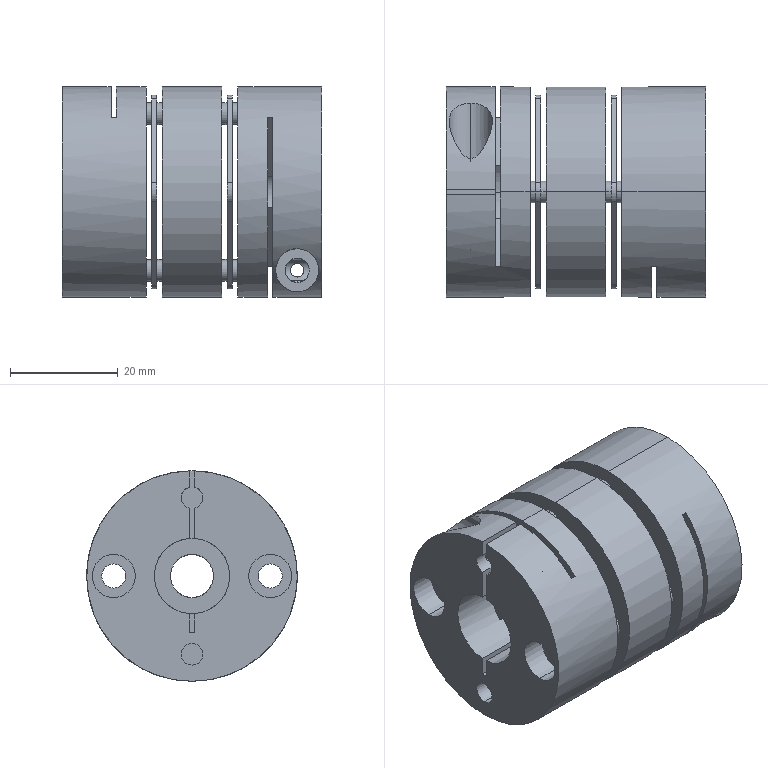Part | STEP file | 1 solid | 155 faces | box 48 x 39 x 39 mm | volume 40714 mm3 | cylinder 96 | plane 51 | cone 8 | commonest cylinder face diameters 4.5 x28 4 x26 8 x14 5 x10 17 x6 39 x6